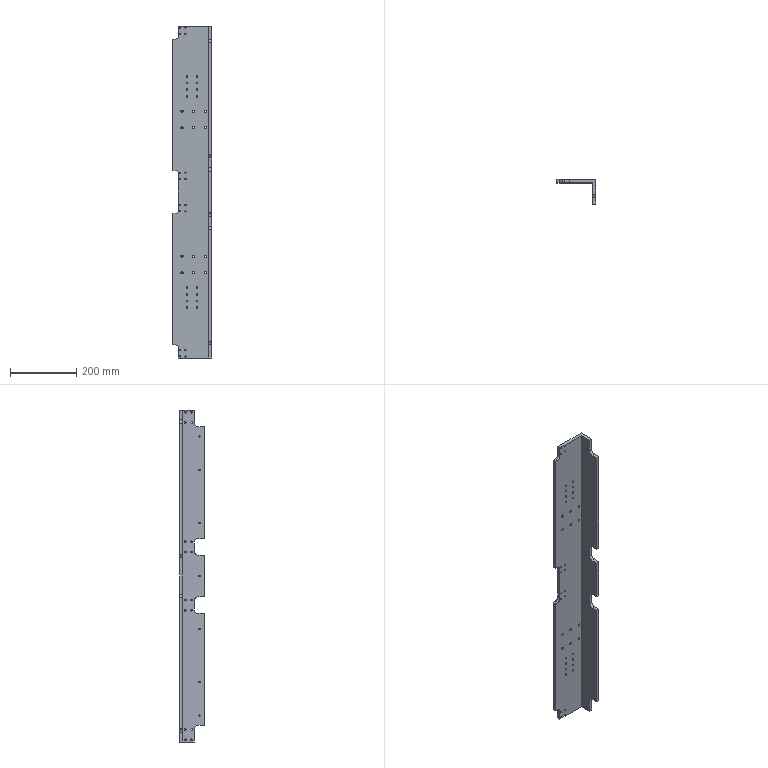Part | SolidWorks | features HoleWzd 5, Cut 2, MoveFace 2, Chamfer 1, Extrusion 1, Fillet 1 | 1 solid | 172 faces | box 120 x 75 x 1000 mm | volume 1739267 mm3 | cylinder 144 | plane 28 | commonest cylinder face diameters 5 x64 3.3 x32 6.8 x24 4.2 x14 20 x10